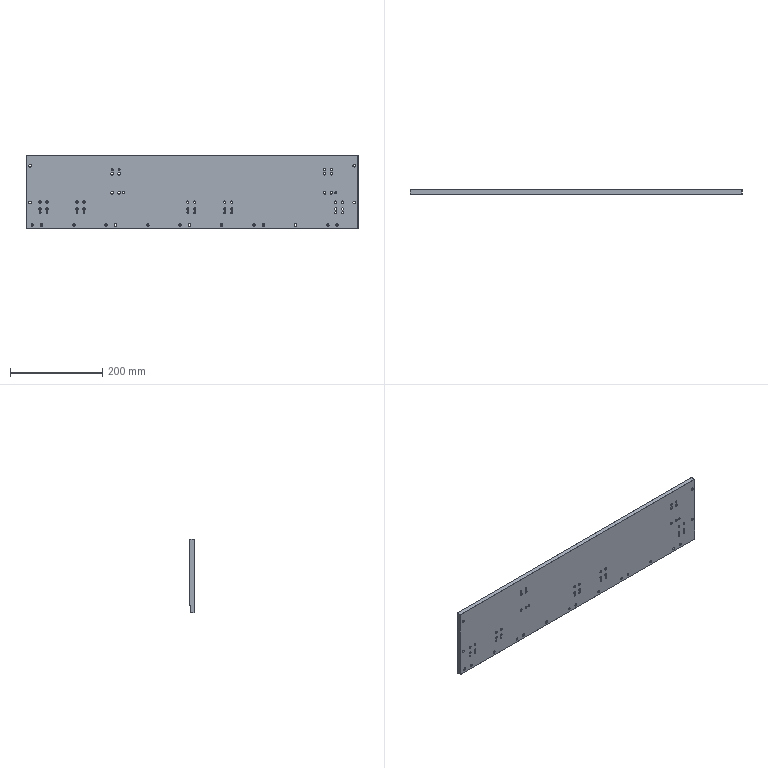Part | NX | 1 solid | 275 faces | box 719 x 10 x 159 mm | volume 1113123 mm3 | cylinder 132 | cone 116 | plane 27 | commonest cylinder face diameters 5 x68 4 x32 5.5 x16 6 x8 10 x8